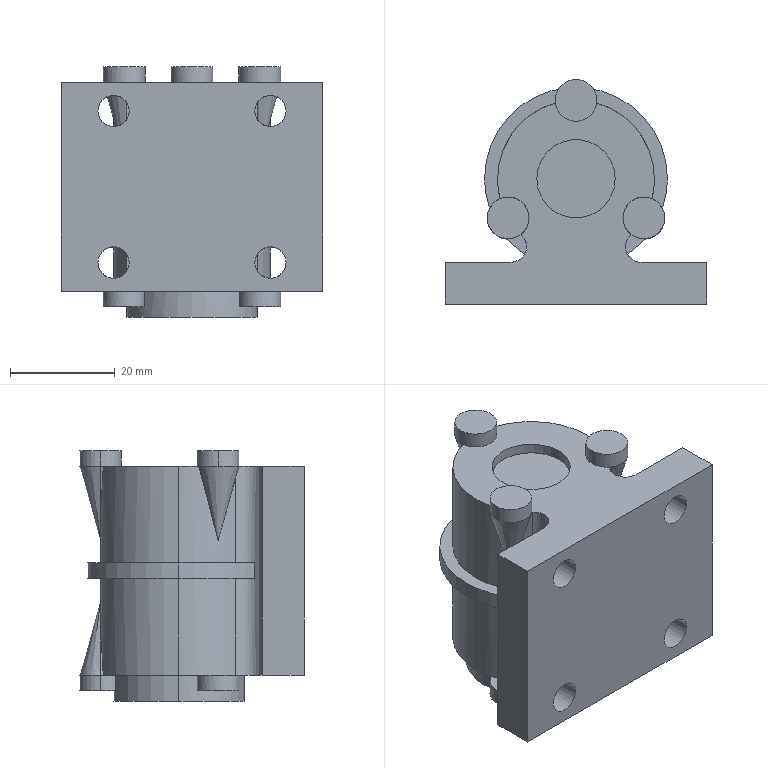Part | SolidWorks | features BaseBody 1 | 1 solid | 74 faces | box 50 x 43 x 48 mm | volume 49165 mm3 | cylinder 37 | plane 25 | cone 12 | commonest cylinder face diameters 6 x12 8 x12 30 x6 35 x3 15 x2 25 x2